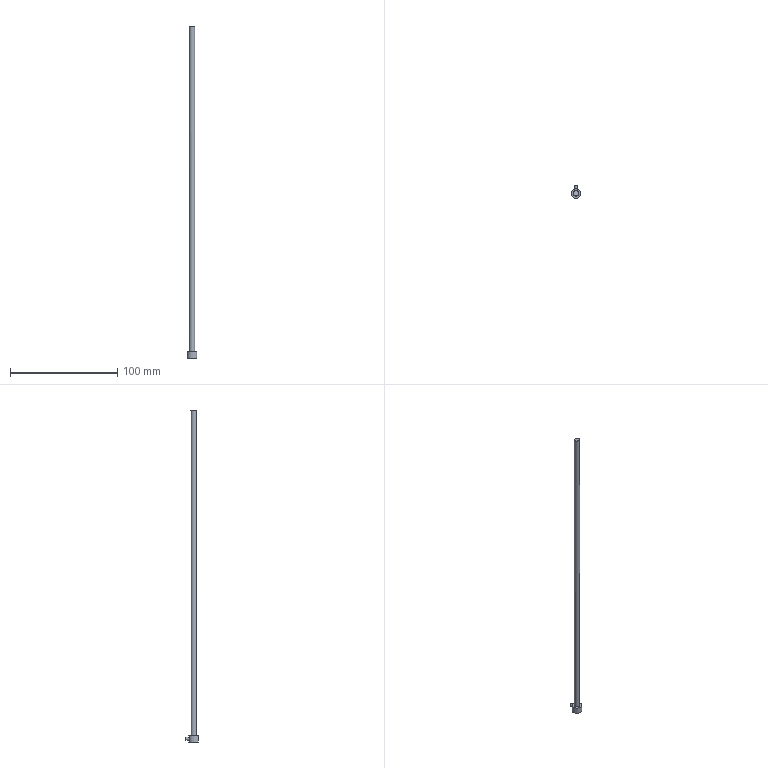Part | STEP file | E105-19-315 | 1 solid | 8 faces | box 9 x 12 x 309.26 mm | volume 6349 mm3 | cylinder 3 | plane 3 | spline 1 | cone 1 | commonest cylinder face diameters 3 x1 5 x1 9 x1
STEP:
#1=CARTESIAN_POINT('',(0.,0.,0.));
#2=DIRECTION('',(0.,0.,1.));
#3=DIRECTION('',(1.,0.,0.));
#4=AXIS2_PLACEMENT_3D('',#1,#2,#3);
#5=CARTESIAN_POINT('',(2.261,-1.066,308.914));
#6=VERTEX_POINT('',#5);
#7=CARTESIAN_POINT('',(-2.5,0.,308.912));
#8=VERTEX_POINT('',#7);
#9=CARTESIAN_POINT('',(2.261,-1.066,308.914));
#10=CARTESIAN_POINT('',(2.141,-1.321,308.963));
#11=CARTESIAN_POINT('',(1.975,-1.558,309.011));
#12=CARTESIAN_POINT('',(1.777,-1.759,309.053));
#13=CARTESIAN_POINT('',(1.578,-1.96,309.095));
#14=CARTESIAN_POINT('',(1.341,-2.129,309.134));
#15=CARTESIAN_POINT('',(1.085,-2.252,309.164));
#16=CARTESIAN_POINT('',(0.8317,-2.374,309.195));
#17=CARTESIAN_POINT('',(0.553,-2.454,309.22));
#18=CARTESIAN_POINT('',(0.2723,-2.485,309.236));
#19=CARTESIAN_POINT('',(-0.004267,-2.515,309.252));
#20=CARTESIAN_POINT('',(-0.2904,-2.499,309.26));
#21=CARTESIAN_POINT('',(-0.562,-2.436,309.26));
#22=CARTESIAN_POINT('',(-0.8311,-2.374,309.26));
#23=CARTESIAN_POINT('',(-1.093,-2.265,309.252));
#24=CARTESIAN_POINT('',(-1.327,-2.119,309.236));
#25=CARTESIAN_POINT('',(-1.561,-1.972,309.22));
#26=CARTESIAN_POINT('',(-1.772,-1.785,309.197));
#27=CARTESIAN_POINT('',(-1.944,-1.571,309.166));
#28=CARTESIAN_POINT('',(-2.118,-1.356,309.136));
#29=CARTESIAN_POINT('',(-2.257,-1.109,309.099));
#30=CARTESIAN_POINT('',(-2.351,-0.8505,309.057));
#31=CARTESIAN_POINT('',(-2.446,-0.588,309.014));
#32=CARTESIAN_POINT('',(-2.497,-0.3065,308.966));
#33=CARTESIAN_POINT('',(-2.5,-0.02854,308.917));
#34=CARTESIAN_POINT('',(-2.503,0.2536,308.866));
#35=CARTESIAN_POINT('',(-2.457,0.5396,308.813));
#36=CARTESIAN_POINT('',(-2.366,0.8063,308.76));
#37=CARTESIAN_POINT('',(-2.275,1.075,308.707));
#38=CARTESIAN_POINT('',(-2.134,1.332,308.654));
#39=CARTESIAN_POINT('',(-1.957,1.556,308.606));
#40=CARTESIAN_POINT('',(-1.78,1.778,308.558));
#41=CARTESIAN_POINT('',(-1.561,1.974,308.512));
#42=CARTESIAN_POINT('',(-1.318,2.124,308.474));
#43=CARTESIAN_POINT('',(-1.078,2.273,308.437));
#44=CARTESIAN_POINT('',(-0.8076,2.383,308.405));
#45=CARTESIAN_POINT('',(-0.53,2.443,308.383));
#46=CARTESIAN_POINT('',(-0.2575,2.502,308.361));
#47=CARTESIAN_POINT('',(0.02984,2.515,308.347));
#48=CARTESIAN_POINT('',(0.3074,2.481,308.343));
#49=CARTESIAN_POINT('',(0.5811,2.447,308.338));
#50=CARTESIAN_POINT('',(0.8529,2.366,308.343));
#51=CARTESIAN_POINT('',(1.1,2.245,308.356));
#52=CARTESIAN_POINT('',(1.347,2.124,308.369));
#53=CARTESIAN_POINT('',(1.576,1.96,308.391));
#54=CARTESIAN_POINT('',(1.769,1.766,308.42));
#55=CARTESIAN_POINT('',(1.964,1.571,308.449));
#56=CARTESIAN_POINT('',(2.128,1.341,308.485));
#57=CARTESIAN_POINT('',(2.248,1.094,308.526));
#58=CARTESIAN_POINT('',(2.37,0.8435,308.567));
#59=CARTESIAN_POINT('',(2.45,0.5692,308.614));
#60=CARTESIAN_POINT('',(2.483,0.2935,308.663));
#61=CARTESIAN_POINT('',(2.516,0.01345,308.712));
#62=CARTESIAN_POINT('',(2.501,-0.2757,308.765));
#63=CARTESIAN_POINT('',(2.439,-0.5505,308.816));
#64=CARTESIAN_POINT('',(2.399,-0.7277,308.849));
#65=CARTESIAN_POINT('',(2.339,-0.9016,308.882));
#66=CARTESIAN_POINT('',(2.261,-1.066,308.914));
#67=B_SPLINE_CURVE_WITH_KNOTS('',3,(#9,#10,#11,#12,#13,#14,#15,#16,#17,#18,#19,#20,#21,#22,#23,#24,#25,#26,#27,#28,#29,#30,#31,#32,#33,#34,#35,#36,#37,#38,#39,#40,#41,#42,#43,#44,#45,#46,#47,#48,#49,#50,#51,#52,#53,#54,#55,#56,#57,#58,#59,#60,#61,#62,#63,#64,#65,#66),.UNSPECIFIED.,.T.,.F.,(1,3,3,3,3,3,3,3,3,3,3,3,3,3,3,3,3,3,3,3,3,1),(-0.03486,0.,0.05436,0.1088,0.1626,0.2156,0.2682,0.3207,0.3737,0.4274,0.4819,0.537,0.592,0.6462,0.6995,0.752,0.8043,0.857,0.9107,0.9651,1.,1.054),.UNSPECIFIED.);
#68=CARTESIAN_POINT('',(0.,0.,106.));
#69=DIRECTION('',(0.,0.,-1.));
#70=DIRECTION('',(-1.,0.,0.));
#71=AXIS2_PLACEMENT_3D('',#68,#69,#70);
#72=CYLINDRICAL_SURFACE('',#71,2.5);
#73=CARTESIAN_POINT('',(3.582,-202.914));
#74=CARTESIAN_POINT('',(3.606,-202.924));
#75=CARTESIAN_POINT('',(3.653,-202.944));
#76=CARTESIAN_POINT('',(3.724,-202.974));
#77=CARTESIAN_POINT('',(3.795,-203.004));
#78=CARTESIAN_POINT('',(3.866,-203.032));
#79=CARTESIAN_POINT('',(3.937,-203.059));
#80=CARTESIAN_POINT('',(4.008,-203.085));
#81=CARTESIAN_POINT('',(4.08,-203.109));
#82=CARTESIAN_POINT('',(4.151,-203.132));
#83=CARTESIAN_POINT('',(4.223,-203.153));
#84=CARTESIAN_POINT('',(4.294,-203.173));
#85=CARTESIAN_POINT('',(4.366,-203.191));
#86=CARTESIAN_POINT('',(4.438,-203.207));
#87=CARTESIAN_POINT('',(4.509,-203.221));
#88=CARTESIAN_POINT('',(4.581,-203.233));
#89=CARTESIAN_POINT('',(4.653,-203.243));
#90=CARTESIAN_POINT('',(4.725,-203.25));
#91=CARTESIAN_POINT('',(4.797,-203.256));
#92=CARTESIAN_POINT('',(4.869,-203.259));
#93=CARTESIAN_POINT('',(4.941,-203.261));
#94=CARTESIAN_POINT('',(5.013,-203.259));
#95=CARTESIAN_POINT('',(5.085,-203.256));
#96=CARTESIAN_POINT('',(5.157,-203.25));
#97=CARTESIAN_POINT('',(5.229,-203.242));
#98=CARTESIAN_POINT('',(5.3,-203.232));
#99=CARTESIAN_POINT('',(5.372,-203.22));
#100=CARTESIAN_POINT('',(5.444,-203.206));
#101=CARTESIAN_POINT('',(5.516,-203.189));
#102=CARTESIAN_POINT('',(5.588,-203.171));
#103=CARTESIAN_POINT('',(5.659,-203.151));
#104=CARTESIAN_POINT('',(5.73,-203.129));
#105=CARTESIAN_POINT('',(5.802,-203.105));
#106=CARTESIAN_POINT('',(5.873,-203.08));
#107=CARTESIAN_POINT('',(5.944,-203.054));
#108=CARTESIAN_POINT('',(6.015,-203.026));
#109=CARTESIAN_POINT('',(6.087,-202.997));
#110=CARTESIAN_POINT('',(6.158,-202.967));
#111=CARTESIAN_POINT('',(6.229,-202.936));
#112=CARTESIAN_POINT('',(6.299,-202.904));
#113=CARTESIAN_POINT('',(6.37,-202.872));
#114=CARTESIAN_POINT('',(6.441,-202.84));
#115=CARTESIAN_POINT('',(6.512,-202.807));
#116=CARTESIAN_POINT('',(6.583,-202.774));
#117=CARTESIAN_POINT('',(6.653,-202.741));
#118=CARTESIAN_POINT('',(6.724,-202.708));
#119=CARTESIAN_POINT('',(6.795,-202.676));
#120=CARTESIAN_POINT('',(6.866,-202.644));
#121=CARTESIAN_POINT('',(6.937,-202.613));
#122=CARTESIAN_POINT('',(7.007,-202.584));
#123=CARTESIAN_POINT('',(7.079,-202.555));
#124=CARTESIAN_POINT('',(7.15,-202.527));
#125=CARTESIAN_POINT('',(7.221,-202.501));
#126=CARTESIAN_POINT('',(7.292,-202.476));
#127=CARTESIAN_POINT('',(7.363,-202.453));
#128=CARTESIAN_POINT('',(7.435,-202.432));
#129=CARTESIAN_POINT('',(7.507,-202.413));
#130=CARTESIAN_POINT('',(7.578,-202.395));
#131=CARTESIAN_POINT('',(7.65,-202.381));
#132=CARTESIAN_POINT('',(7.722,-202.368));
#133=CARTESIAN_POINT('',(7.794,-202.358));
#134=CARTESIAN_POINT('',(7.866,-202.35));
#135=CARTESIAN_POINT('',(7.938,-202.344));
#136=CARTESIAN_POINT('',(8.009,-202.341));
#137=CARTESIAN_POINT('',(8.081,-202.341));
#138=CARTESIAN_POINT('',(8.153,-202.343));
#139=CARTESIAN_POINT('',(8.226,-202.347));
#140=CARTESIAN_POINT('',(8.297,-202.354));
#141=CARTESIAN_POINT('',(8.369,-202.364));
#142=CARTESIAN_POINT('',(8.441,-202.375));
#143=CARTESIAN_POINT('',(8.513,-202.389));
#144=CARTESIAN_POINT('',(8.585,-202.406));
#145=CARTESIAN_POINT('',(8.656,-202.424));
#146=CARTESIAN_POINT('',(8.728,-202.444));
#147=CARTESIAN_POINT('',(8.799,-202.466));
#148=CARTESIAN_POINT('',(8.871,-202.49));
#149=CARTESIAN_POINT('',(8.942,-202.515));
#150=CARTESIAN_POINT('',(9.013,-202.541));
#151=CARTESIAN_POINT('',(9.084,-202.569));
#152=CARTESIAN_POINT('',(9.155,-202.598));
#153=CARTESIAN_POINT('',(9.227,-202.628));
#154=CARTESIAN_POINT('',(9.297,-202.658));
#155=CARTESIAN_POINT('',(9.368,-202.69));
#156=CARTESIAN_POINT('',(9.439,-202.721));
#157=CARTESIAN_POINT('',(9.51,-202.754));
#158=CARTESIAN_POINT('',(9.581,-202.786));
#159=CARTESIAN_POINT('',(9.651,-202.818));
#160=CARTESIAN_POINT('',(9.723,-202.85));
#161=CARTESIAN_POINT('',(9.794,-202.882));
#162=CARTESIAN_POINT('',(9.842,-202.903));
#163=CARTESIAN_POINT('',(9.865,-202.914));
#164=B_SPLINE_CURVE_WITH_KNOTS('',3,(#73,#74,#75,#76,#77,#78,#79,#80,#81,#82,#83,#84,#85,#86,#87,#88,#89,#90,#91,#92,#93,#94,#95,#96,#97,#98,#99,#100,#101,#102,#103,#104,#105,#106,#107,#108,#109,#110,#111,#112,#113,#114,#115,#116,#117,#118,#119,#120,#121,#122,#123,#124,#125,#126,#127,#128,#129,#130,#131,#132,#133,#134,#135,#136,#137,#138,#139,#140,#141,#142,#143,#144,#145,#146,#147,#148,#149,#150,#151,#152,#153,#154,#155,#156,#157,#158,#159,#160,#161,#162,#163),.UNSPECIFIED.,.F.,.F.,(4,1,1,1,1,1,1,1,1,1,1,1,1,1,1,1,1,1,1,1,1,1,1,1,1,1,1,1,1,1,1,1,1,1,1,1,1,1,1,1,1,1,1,1,1,1,1,1,1,1,1,1,1,1,1,1,1,1,1,1,1,1,1,1,1,1,1,1,1,1,1,1,1,1,1,1,1,1,1,1,1,1,1,1,1,1,1,1,4),(0.,0.01136,0.02273,0.03409,0.04545,0.05682,0.06818,0.07955,0.09091,0.1023,0.1136,0.125,0.1364,0.1477,0.1591,0.1705,0.1818,0.1932,0.2045,0.2159,0.2273,0.2386,0.25,0.2614,0.2727,0.2841,0.2955,0.3068,0.3182,0.3295,0.3409,0.3523,0.3636,0.375,0.3864,0.3977,0.4091,0.4205,0.4318,0.4432,0.4545,0.4659,0.4773,0.4886,0.5,0.5114,0.5227,0.5341,0.5455,0.5568,0.5682,0.5795,0.5909,0.6023,0.6136,0.625,0.6364,0.6477,0.6591,0.6705,0.6818,0.6932,0.7045,0.7159,0.7273,0.7386,0.75,0.7614,0.7727,0.7841,0.7955,0.8068,0.8182,0.8295,0.8409,0.8523,0.8636,0.875,0.8864,0.8977,0.9091,0.9205,0.9318,0.9432,0.9545,0.9659,0.9773,0.9886,1.),.QUASI_UNIFORM_KNOTS.);
#165=(GEOMETRIC_REPRESENTATION_CONTEXT(2)PARAMETRIC_REPRESENTATION_CONTEXT()REPRESENTATION_CONTEXT('',''));
#166=DEFINITIONAL_REPRESENTATION('',(#164),#165);
#167=PCURVE('',#72,#166);
#168=CARTESIAN_POINT('',(-6.353,3.18,308.471));
#169=CARTESIAN_POINT('',(-6.352,0.7834,308.933));
#170=CARTESIAN_POINT('',(-6.351,-1.62,309.36));
#171=CARTESIAN_POINT('',(-6.35,-4.031,309.75));
#172=CARTESIAN_POINT('',(-1.324,3.172,308.275));
#173=CARTESIAN_POINT('',(-1.323,0.7765,308.737));
#174=CARTESIAN_POINT('',(-1.322,-1.626,309.164));
#175=CARTESIAN_POINT('',(-1.32,-4.035,309.555));
#176=CARTESIAN_POINT('',(3.706,3.167,308.077));
#177=CARTESIAN_POINT('',(3.707,0.7722,308.54));
#178=CARTESIAN_POINT('',(3.708,-1.629,308.967));
#179=CARTESIAN_POINT('',(3.709,-4.037,309.359));
#180=CARTESIAN_POINT('',(8.735,3.164,307.878));
#181=CARTESIAN_POINT('',(8.736,0.7703,308.342));
#182=CARTESIAN_POINT('',(8.737,-1.63,308.769));
#183=CARTESIAN_POINT('',(8.738,-4.037,309.161));
#184=B_SPLINE_SURFACE_WITH_KNOTS('',3,3,((#168,#169,#170,#171),(#172,#173,#174,#175),(#176,#177,#178,#179),(#180,#181,#182,#183)),.UNSPECIFIED.,.F.,.F.,.F.,(4,4),(4,4),(0.,1.),(0.,1.),.PIECEWISE_BEZIER_KNOTS.);
#185=CARTESIAN_POINT('',(0.5708,0.5885));
#186=CARTESIAN_POINT('',(0.5694,0.5948));
#187=CARTESIAN_POINT('',(0.5663,0.6074));
#188=CARTESIAN_POINT('',(0.5612,0.6256));
#189=CARTESIAN_POINT('',(0.5555,0.6432));
#190=CARTESIAN_POINT('',(0.5494,0.66));
#191=CARTESIAN_POINT('',(0.5427,0.676));
#192=CARTESIAN_POINT('',(0.5357,0.6911));
#193=CARTESIAN_POINT('',(0.5281,0.7053));
#194=CARTESIAN_POINT('',(0.5202,0.7185));
#195=CARTESIAN_POINT('',(0.5118,0.7307));
#196=CARTESIAN_POINT('',(0.5032,0.7419));
#197=CARTESIAN_POINT('',(0.4942,0.7519));
#198=CARTESIAN_POINT('',(0.485,0.7607));
#199=CARTESIAN_POINT('',(0.4754,0.7683));
#200=CARTESIAN_POINT('',(0.4657,0.7747));
#201=CARTESIAN_POINT('',(0.4557,0.7799));
#202=CARTESIAN_POINT('',(0.4457,0.7837));
#203=CARTESIAN_POINT('',(0.4356,0.7863));
#204=CARTESIAN_POINT('',(0.4254,0.7875));
#205=CARTESIAN_POINT('',(0.4151,0.7874));
#206=CARTESIAN_POINT('',(0.4049,0.786));
#207=CARTESIAN_POINT('',(0.3947,0.7833));
#208=CARTESIAN_POINT('',(0.3847,0.7794));
#209=CARTESIAN_POINT('',(0.3748,0.7741));
#210=CARTESIAN_POINT('',(0.365,0.7675));
#211=CARTESIAN_POINT('',(0.3555,0.7596));
#212=CARTESIAN_POINT('',(0.3462,0.7506));
#213=CARTESIAN_POINT('',(0.3372,0.7404));
#214=CARTESIAN_POINT('',(0.3286,0.7291));
#215=CARTESIAN_POINT('',(0.3203,0.7166));
#216=CARTESIAN_POINT('',(0.3123,0.7031));
#217=CARTESIAN_POINT('',(0.3048,0.6886));
#218=CARTESIAN_POINT('',(0.2978,0.6733));
#219=CARTESIAN_POINT('',(0.2912,0.6571));
#220=CARTESIAN_POINT('',(0.2851,0.6401));
#221=CARTESIAN_POINT('',(0.2796,0.6223));
#222=CARTESIAN_POINT('',(0.2745,0.6038));
#223=CARTESIAN_POINT('',(0.27,0.5847));
#224=CARTESIAN_POINT('',(0.2661,0.5652));
#225=CARTESIAN_POINT('',(0.2628,0.5452));
#226=CARTESIAN_POINT('',(0.2601,0.5249));
#227=CARTESIAN_POINT('',(0.2579,0.5041));
#228=CARTESIAN_POINT('',(0.2564,0.4832));
#229=CARTESIAN_POINT('',(0.2555,0.4621));
#230=CARTESIAN_POINT('',(0.2553,0.4481));
#231=CARTESIAN_POINT('',(0.2553,0.4411));
#232=B_SPLINE_CURVE_WITH_KNOTS('',3,(#185,#186,#187,#188,#189,#190,#191,#192,#193,#194,#195,#196,#197,#198,#199,#200,#201,#202,#203,#204,#205,#206,#207,#208,#209,#210,#211,#212,#213,#214,#215,#216,#217,#218,#219,#220,#221,#222,#223,#224,#225,#226,#227,#228,#229,#230,#231),.UNSPECIFIED.,.F.,.F.,(4,1,1,1,1,1,1,1,1,1,1,1,1,1,1,1,1,1,1,1,1,1,1,1,1,1,1,1,1,1,1,1,1,1,1,1,1,1,1,1,1,1,1,1,4),(0.,0.009755,0.01951,0.02927,0.03902,0.04878,0.05853,0.06829,0.07804,0.0878,0.09755,0.1073,0.1171,0.1268,0.1366,0.1463,0.1561,0.1658,0.1756,0.1853,0.1951,0.2049,0.2146,0.2244,0.2341,0.2439,0.2536,0.2634,0.2731,0.2829,0.2927,0.3024,0.3122,0.3219,0.3317,0.3414,0.3512,0.3609,0.3707,0.3804,0.3902,0.4,0.4097,0.4195,0.4292),.QUASI_UNIFORM_KNOTS.);
#233=(GEOMETRIC_REPRESENTATION_CONTEXT(2)PARAMETRIC_REPRESENTATION_CONTEXT()REPRESENTATION_CONTEXT('',''));
#234=DEFINITIONAL_REPRESENTATION('',(#232),#233);
#235=PCURVE('',#184,#234);
#236=SURFACE_CURVE('',#67,(#167,#235),.PCURVE_S1.);
#237=EDGE_CURVE('',#6,#8,#236,.T.);
#238=ORIENTED_EDGE('',*,*,#237,.T.);
#239=CARTESIAN_POINT('',(-2.5,0.,6.));
#240=VERTEX_POINT('',#239);
#241=CARTESIAN_POINT('',(-2.5,0.,308.912));
#242=CARTESIAN_POINT('',(-2.5,0.,6.));
#243=B_SPLINE_CURVE_WITH_KNOTS('',1,(#241,#242),.UNSPECIFIED.,.F.,.F.,(2,2),(-202.912,100.),.PIECEWISE_BEZIER_KNOTS.);
#244=CARTESIAN_POINT('',(6.283,0.));
#245=DIRECTION('',(0.,1.));
#246=VECTOR('',#245,1.);
#247=LINE('',#244,#246);
#248=(GEOMETRIC_REPRESENTATION_CONTEXT(2)PARAMETRIC_REPRESENTATION_CONTEXT()REPRESENTATION_CONTEXT('',''));
#249=DEFINITIONAL_REPRESENTATION('',(#247),#248);
#250=PCURVE('',#72,#249);
#251=CARTESIAN_POINT('',(0.,0.));
#252=DIRECTION('',(0.,1.));
#253=VECTOR('',#252,1.);
#254=LINE('',#251,#253);
#255=(GEOMETRIC_REPRESENTATION_CONTEXT(2)PARAMETRIC_REPRESENTATION_CONTEXT()REPRESENTATION_CONTEXT('',''));
#256=DEFINITIONAL_REPRESENTATION('',(#254),#255);
#257=PCURVE('',#72,#256);
#258=SEAM_CURVE('',#243,(#250,#257),.PCURVE_S1.);
#259=EDGE_CURVE('',#8,#240,#258,.T.);
#260=ORIENTED_EDGE('',*,*,#259,.T.);
#261=CARTESIAN_POINT('',(0.,0.,6.));
#262=DIRECTION('',(0.,0.,-1.));
#263=DIRECTION('',(-1.,0.,0.));
#264=AXIS2_PLACEMENT_3D('',#261,#262,#263);
#265=CIRCLE('',#264,2.5);
#266=CARTESIAN_POINT('',(0.,100.));
#267=DIRECTION('',(1.,0.));
#268=VECTOR('',#267,1.);
#269=LINE('',#266,#268);
#270=(GEOMETRIC_REPRESENTATION_CONTEXT(2)PARAMETRIC_REPRESENTATION_CONTEXT()REPRESENTATION_CONTEXT('',''));
#271=DEFINITIONAL_REPRESENTATION('',(#269),#270);
#272=PCURVE('',#72,#271);
#273=CARTESIAN_POINT('',(0.,0.,6.));
#274=DIRECTION('',(0.,0.,-1.));
#275=DIRECTION('',(1.,0.,0.));
#276=AXIS2_PLACEMENT_3D('',#273,#274,#275);
#277=PLANE('',#276);
#278=CARTESIAN_POINT('',(0.,0.));
#279=DIRECTION('',(-1.,0.));
#280=AXIS2_PLACEMENT_2D('',#278,#279);
#281=CIRCLE('',#280,2.5);
#282=(GEOMETRIC_REPRESENTATION_CONTEXT(2)PARAMETRIC_REPRESENTATION_CONTEXT()REPRESENTATION_CONTEXT('',''));
#283=DEFINITIONAL_REPRESENTATION('',(#281),#282);
#284=PCURVE('',#277,#283);
#285=SURFACE_CURVE('',#265,(#272,#284),.PCURVE_S1.);
#286=EDGE_CURVE('',#240,#240,#285,.T.);
#287=ORIENTED_EDGE('',*,*,#286,.F.);
#288=ORIENTED_EDGE('',*,*,#259,.F.);
#289=CARTESIAN_POINT('',(2.261,-1.066,308.914));
#290=CARTESIAN_POINT('',(2.141,-1.321,308.963));
#291=CARTESIAN_POINT('',(1.975,-1.558,309.011));
#292=CARTESIAN_POINT('',(1.777,-1.759,309.053));
#293=CARTESIAN_POINT('',(1.578,-1.96,309.095));
#294=CARTESIAN_POINT('',(1.341,-2.129,309.134));
#295=CARTESIAN_POINT('',(1.085,-2.252,309.164));
#296=CARTESIAN_POINT('',(0.8317,-2.374,309.195));
#297=CARTESIAN_POINT('',(0.553,-2.454,309.22));
#298=CARTESIAN_POINT('',(0.2723,-2.485,309.236));
#299=CARTESIAN_POINT('',(-0.004267,-2.515,309.252));
#300=CARTESIAN_POINT('',(-0.2904,-2.499,309.26));
#301=CARTESIAN_POINT('',(-0.562,-2.436,309.26));
#302=CARTESIAN_POINT('',(-0.8311,-2.374,309.26));
#303=CARTESIAN_POINT('',(-1.093,-2.265,309.252));
#304=CARTESIAN_POINT('',(-1.327,-2.119,309.236));
#305=CARTESIAN_POINT('',(-1.561,-1.972,309.22));
#306=CARTESIAN_POINT('',(-1.772,-1.785,309.197));
#307=CARTESIAN_POINT('',(-1.944,-1.571,309.166));
#308=CARTESIAN_POINT('',(-2.118,-1.356,309.136));
#309=CARTESIAN_POINT('',(-2.257,-1.109,309.099));
#310=CARTESIAN_POINT('',(-2.351,-0.8505,309.057));
#311=CARTESIAN_POINT('',(-2.446,-0.588,309.014));
#312=CARTESIAN_POINT('',(-2.497,-0.3065,308.966));
#313=CARTESIAN_POINT('',(-2.5,-0.02854,308.917));
#314=CARTESIAN_POINT('',(-2.503,0.2536,308.866));
#315=CARTESIAN_POINT('',(-2.457,0.5396,308.813));
#316=CARTESIAN_POINT('',(-2.366,0.8063,308.76));
#317=CARTESIAN_POINT('',(-2.275,1.075,308.707));
#318=CARTESIAN_POINT('',(-2.134,1.332,308.654));
#319=CARTESIAN_POINT('',(-1.957,1.556,308.606));
#320=CARTESIAN_POINT('',(-1.78,1.778,308.558));
#321=CARTESIAN_POINT('',(-1.561,1.974,308.512));
#322=CARTESIAN_POINT('',(-1.318,2.124,308.474));
#323=CARTESIAN_POINT('',(-1.078,2.273,308.437));
#324=CARTESIAN_POINT('',(-0.8076,2.383,308.405));
#325=CARTESIAN_POINT('',(-0.53,2.443,308.383));
#326=CARTESIAN_POINT('',(-0.2575,2.502,308.361));
#327=CARTESIAN_POINT('',(0.02984,2.515,308.347));
#328=CARTESIAN_POINT('',(0.3074,2.481,308.343));
#329=CARTESIAN_POINT('',(0.5811,2.447,308.338));
#330=CARTESIAN_POINT('',(0.8529,2.366,308.343));
#331=CARTESIAN_POINT('',(1.1,2.245,308.356));
#332=CARTESIAN_POINT('',(1.347,2.124,308.369));
#333=CARTESIAN_POINT('',(1.576,1.96,308.391));
#334=CARTESIAN_POINT('',(1.769,1.766,308.42));
#335=CARTESIAN_POINT('',(1.964,1.571,308.449));
#336=CARTESIAN_POINT('',(2.128,1.341,308.485));
#337=CARTESIAN_POINT('',(2.248,1.094,308.526));
#338=CARTESIAN_POINT('',(2.37,0.8435,308.567));
#339=CARTESIAN_POINT('',(2.45,0.5692,308.614));
#340=CARTESIAN_POINT('',(2.483,0.2935,308.663));
#341=CARTESIAN_POINT('',(2.516,0.01345,308.712));
#342=CARTESIAN_POINT('',(2.501,-0.2757,308.765));
#343=CARTESIAN_POINT('',(2.439,-0.5505,308.816));
#344=CARTESIAN_POINT('',(2.399,-0.7277,308.849));
#345=CARTESIAN_POINT('',(2.339,-0.9016,308.882));
#346=CARTESIAN_POINT('',(2.261,-1.066,308.914));
#347=B_SPLINE_CURVE_WITH_KNOTS('',3,(#289,#290,#291,#292,#293,#294,#295,#296,#297,#298,#299,#300,#301,#302,#303,#304,#305,#306,#307,#308,#309,#310,#311,#312,#313,#314,#315,#316,#317,#318,#319,#320,#321,#322,#323,#324,#325,#326,#327,#328,#329,#330,#331,#332,#333,#334,#335,#336,#337,#338,#339,#340,#341,#342,#343,#344,#345,#346),.UNSPECIFIED.,.T.,.F.,(1,3,3,3,3,3,3,3,3,3,3,3,3,3,3,3,3,3,3,3,3,1),(-0.03486,0.,0.05436,0.1088,0.1626,0.2156,0.2682,0.3207,0.3737,0.4274,0.4819,0.537,0.592,0.6462,0.6995,0.752,0.8043,0.857,0.9107,0.9651,1.,1.054),.UNSPECIFIED.);
#348=CARTESIAN_POINT('',(-2.701,-202.914));
#349=CARTESIAN_POINT('',(-2.677,-202.924));
#350=CARTESIAN_POINT('',(-2.63,-202.944));
#351=CARTESIAN_POINT('',(-2.559,-202.974));
#352=CARTESIAN_POINT('',(-2.488,-203.004));
#353=CARTESIAN_POINT('',(-2.417,-203.032));
#354=CARTESIAN_POINT('',(-2.346,-203.059));
#355=CARTESIAN_POINT('',(-2.275,-203.085));
#356=CARTESIAN_POINT('',(-2.203,-203.109));
#357=CARTESIAN_POINT('',(-2.132,-203.132));
#358=CARTESIAN_POINT('',(-2.06,-203.153));
#359=CARTESIAN_POINT('',(-1.989,-203.173));
#360=CARTESIAN_POINT('',(-1.918,-203.191));
#361=CARTESIAN_POINT('',(-1.846,-203.207));
#362=CARTESIAN_POINT('',(-1.774,-203.221));
#363=CARTESIAN_POINT('',(-1.702,-203.233));
#364=CARTESIAN_POINT('',(-1.63,-203.243));
#365=CARTESIAN_POINT('',(-1.558,-203.25));
#366=CARTESIAN_POINT('',(-1.486,-203.256));
#367=CARTESIAN_POINT('',(-1.414,-203.259));
#368=CARTESIAN_POINT('',(-1.342,-203.261));
#369=CARTESIAN_POINT('',(-1.271,-203.259));
#370=CARTESIAN_POINT('',(-1.198,-203.256));
#371=CARTESIAN_POINT('',(-1.126,-203.25));
#372=CARTESIAN_POINT('',(-1.054,-203.242));
#373=CARTESIAN_POINT('',(-0.9828,-203.232));
#374=CARTESIAN_POINT('',(-0.9109,-203.22));
#375=CARTESIAN_POINT('',(-0.839,-203.206));
#376=CARTESIAN_POINT('',(-0.7671,-203.189));
#377=CARTESIAN_POINT('',(-0.6955,-203.171));
#378=CARTESIAN_POINT('',(-0.6243,-203.151));
#379=CARTESIAN_POINT('',(-0.5527,-203.129));
#380=CARTESIAN_POINT('',(-0.4812,-203.105));
#381=CARTESIAN_POINT('',(-0.4097,-203.08));
#382=CARTESIAN_POINT('',(-0.3388,-203.054));
#383=CARTESIAN_POINT('',(-0.2678,-203.026));
#384=CARTESIAN_POINT('',(-0.1966,-202.997));
#385=CARTESIAN_POINT('',(-0.1254,-202.967));
#386=CARTESIAN_POINT('',(-0.05444,-202.936));
#387=CARTESIAN_POINT('',(0.01607,-202.904));
#388=CARTESIAN_POINT('',(0.08688,-202.872));
#389=CARTESIAN_POINT('',(0.1578,-202.84));
#390=CARTESIAN_POINT('',(0.2288,-202.807));
#391=CARTESIAN_POINT('',(0.2995,-202.774));
#392=CARTESIAN_POINT('',(0.3699,-202.741));
#393=CARTESIAN_POINT('',(0.4408,-202.708));
#394=CARTESIAN_POINT('',(0.5117,-202.676));
#395=CARTESIAN_POINT('',(0.5827,-202.644));
#396=CARTESIAN_POINT('',(0.6536,-202.613));
#397=CARTESIAN_POINT('',(0.7242,-202.584));
#398=CARTESIAN_POINT('',(0.7953,-202.555));
#399=CARTESIAN_POINT('',(0.8666,-202.527));
#400=CARTESIAN_POINT('',(0.9379,-202.501));
#401=CARTESIAN_POINT('',(1.009,-202.476));
#402=CARTESIAN_POINT('',(1.08,-202.453));
#403=CARTESIAN_POINT('',(1.152,-202.432));
#404=CARTESIAN_POINT('',(1.224,-202.413));
#405=CARTESIAN_POINT('',(1.295,-202.395));
#406=CARTESIAN_POINT('',(1.367,-202.381));
#407=CARTESIAN_POINT('',(1.438,-202.368));
#408=CARTESIAN_POINT('',(1.51,-202.358));
#409=CARTESIAN_POINT('',(1.582,-202.35));
#410=CARTESIAN_POINT('',(1.654,-202.344));
#411=CARTESIAN_POINT('',(1.726,-202.341));
#412=CARTESIAN_POINT('',(1.798,-202.341));
#413=CARTESIAN_POINT('',(1.87,-202.343));
#414=CARTESIAN_POINT('',(1.942,-202.347));
#415=CARTESIAN_POINT('',(2.014,-202.354));
#416=CARTESIAN_POINT('',(2.086,-202.364));
#417=CARTESIAN_POINT('',(2.158,-202.375));
#418=CARTESIAN_POINT('',(2.23,-202.389));
#419=CARTESIAN_POINT('',(2.302,-202.406));
#420=CARTESIAN_POINT('',(2.373,-202.424));
#421=CARTESIAN_POINT('',(2.444,-202.444));
#422=CARTESIAN_POINT('',(2.516,-202.466));
#423=CARTESIAN_POINT('',(2.588,-202.49));
#424=CARTESIAN_POINT('',(2.659,-202.515));
#425=CARTESIAN_POINT('',(2.73,-202.541));
#426=CARTESIAN_POINT('',(2.801,-202.569));
#427=CARTESIAN_POINT('',(2.872,-202.598));
#428=CARTESIAN_POINT('',(2.943,-202.628));
#429=CARTESIAN_POINT('',(3.014,-202.658));
#430=CARTESIAN_POINT('',(3.085,-202.69));
#431=CARTESIAN_POINT('',(3.156,-202.721));
#432=CARTESIAN_POINT('',(3.227,-202.754));
#433=CARTESIAN_POINT('',(3.298,-202.786));
#434=CARTESIAN_POINT('',(3.368,-202.818));
#435=CARTESIAN_POINT('',(3.44,-202.85));
#436=CARTESIAN_POINT('',(3.511,-202.882));
#437=CARTESIAN_POINT('',(3.558,-202.903));
#438=CARTESIAN_POINT('',(3.582,-202.914));
#439=B_SPLINE_CURVE_WITH_KNOTS('',3,(#348,#349,#350,#351,#352,#353,#354,#355,#356,#357,#358,#359,#360,#361,#362,#363,#364,#365,#366,#367,#368,#369,#370,#371,#372,#373,#374,#375,#376,#377,#378,#379,#380,#381,#382,#383,#384,#385,#386,#387,#388,#389,#390,#391,#392,#393,#394,#395,#396,#397,#398,#399,#400,#401,#402,#403,#404,#405,#406,#407,#408,#409,#410,#411,#412,#413,#414,#415,#416,#417,#418,#419,#420,#421,#422,#423,#424,#425,#426,#427,#428,#429,#430,#431,#432,#433,#434,#435,#436,#437,#438),.UNSPECIFIED.,.F.,.F.,(4,1,1,1,1,1,1,1,1,1,1,1,1,1,1,1,1,1,1,1,1,1,1,1,1,1,1,1,1,1,1,1,1,1,1,1,1,1,1,1,1,1,1,1,1,1,1,1,1,1,1,1,1,1,1,1,1,1,1,1,1,1,1,1,1,1,1,1,1,1,1,1,1,1,1,1,1,1,1,1,1,1,1,1,1,1,1,1,4),(0.,0.01136,0.02273,0.03409,0.04545,0.05682,0.06818,0.07955,0.09091,0.1023,0.1136,0.125,0.1364,0.1477,0.1591,0.1705,0.1818,0.1932,0.2045,0.2159,0.2273,0.2386,0.25,0.2614,0.2727,0.2841,0.2955,0.3068,0.3182,0.3295,0.3409,0.3523,0.3636,0.375,0.3864,0.3977,0.4091,0.4205,0.4318,0.4432,0.4545,0.4659,0.4773,0.4886,0.5,0.5114,0.5227,0.5341,0.5455,0.5568,0.5682,0.5795,0.5909,0.6023,0.6136,0.625,0.6364,0.6477,0.6591,0.6705,0.6818,0.6932,0.7045,0.7159,0.7273,0.7386,0.75,0.7614,0.7727,0.7841,0.7955,0.8068,0.8182,0.8295,0.8409,0.8523,0.8636,0.875,0.8864,0.8977,0.9091,0.9205,0.9318,0.9432,0.9545,0.9659,0.9773,0.9886,1.),.QUASI_UNIFORM_KNOTS.);
#440=(GEOMETRIC_REPRESENTATION_CONTEXT(2)PARAMETRIC_REPRESENTATION_CONTEXT()REPRESENTATION_CONTEXT('',''));
#441=DEFINITIONAL_REPRESENTATION('',(#439),#440);
#442=PCURVE('',#72,#441);
#443=CARTESIAN_POINT('',(0.2553,0.4411));
#444=CARTESIAN_POINT('',(0.2553,0.4318));
#445=CARTESIAN_POINT('',(0.2557,0.4131));
#446=CARTESIAN_POINT('',(0.2573,0.3852));
#447=CARTESIAN_POINT('',(0.26,0.3576));
#448=CARTESIAN_POINT('',(0.2637,0.3307));
#449=CARTESIAN_POINT('',(0.2685,0.3046));
#450=CARTESIAN_POINT('',(0.2743,0.2791));
#451=CARTESIAN_POINT('',(0.281,0.2548));
#452=CARTESIAN_POINT('',(0.2886,0.2316));
#453=CARTESIAN_POINT('',(0.2971,0.2099));
#454=CARTESIAN_POINT('',(0.3065,0.1896));
#455=CARTESIAN_POINT('',(0.3166,0.1709));
#456=CARTESIAN_POINT('',(0.3275,0.1539));
#457=CARTESIAN_POINT('',(0.3389,0.139));
#458=CARTESIAN_POINT('',(0.3509,0.1259));
#459=CARTESIAN_POINT('',(0.3634,0.1149));
#460=CARTESIAN_POINT('',(0.3763,0.106));
#461=CARTESIAN_POINT('',(0.3895,0.09947));
#462=CARTESIAN_POINT('',(0.4029,0.0952));
#463=CARTESIAN_POINT('',(0.4165,0.09322));
#464=CARTESIAN_POINT('',(0.4302,0.09356));
#465=CARTESIAN_POINT('',(0.4437,0.09624));
#466=CARTESIAN_POINT('',(0.4571,0.1013));
#467=CARTESIAN_POINT('',(0.4703,0.1087));
#468=CARTESIAN_POINT('',(0.4832,0.1182));
#469=CARTESIAN_POINT('',(0.4955,0.1299));
#470=CARTESIAN_POINT('',(0.5074,0.1438));
#471=CARTESIAN_POINT('',(0.5187,0.1596));
#472=CARTESIAN_POINT('',(0.5294,0.1774));
#473=CARTESIAN_POINT('',(0.5393,0.1967));
#474=CARTESIAN_POINT('',(0.5483,0.2177));
#475=CARTESIAN_POINT('',(0.5566,0.2403));
#476=CARTESIAN_POINT('',(0.5639,0.2641));
#477=CARTESIAN_POINT('',(0.5703,0.2889));
#478=CARTESIAN_POINT('',(0.5756,0.3148));
#479=CARTESIAN_POINT('',(0.58,0.3415));
#480=CARTESIAN_POINT('',(0.5833,0.3689));
#481=CARTESIAN_POINT('',(0.5855,0.3966));
#482=CARTESIAN_POINT('',(0.5867,0.4245));
#483=CARTESIAN_POINT('',(0.5867,0.4527));
#484=CARTESIAN_POINT('',(0.5857,0.4808));
#485=CARTESIAN_POINT('',(0.5836,0.5084));
#486=CARTESIAN_POINT('',(0.5805,0.5358));
#487=CARTESIAN_POINT('',(0.5762,0.5627));
#488=CARTESIAN_POINT('',(0.5727,0.58));
#489=CARTESIAN_POINT('',(0.5708,0.5885));
#490=B_SPLINE_CURVE_WITH_KNOTS('',3,(#443,#444,#445,#446,#447,#448,#449,#450,#451,#452,#453,#454,#455,#456,#457,#458,#459,#460,#461,#462,#463,#464,#465,#466,#467,#468,#469,#470,#471,#472,#473,#474,#475,#476,#477,#478,#479,#480,#481,#482,#483,#484,#485,#486,#487,#488,#489),.UNSPECIFIED.,.F.,.F.,(4,1,1,1,1,1,1,1,1,1,1,1,1,1,1,1,1,1,1,1,1,1,1,1,1,1,1,1,1,1,1,1,1,1,1,1,1,1,1,1,1,1,1,1,4),(0.4292,0.4422,0.4552,0.4681,0.4811,0.4941,0.5071,0.52,0.533,0.546,0.5589,0.5719,0.5849,0.5979,0.6108,0.6238,0.6368,0.6498,0.6627,0.6757,0.6887,0.7016,0.7146,0.7276,0.7406,0.7535,0.7665,0.7795,0.7924,0.8054,0.8184,0.8314,0.8443,0.8573,0.8703,0.8833,0.8962,0.9092,0.9222,0.9351,0.9481,0.9611,0.9741,0.987,1.),.QUASI_UNIFORM_KNOTS.);
#491=(GEOMETRIC_REPRESENTATION_CONTEXT(2)PARAMETRIC_REPRESENTATION_CONTEXT()REPRESENTATION_CONTEXT('',''));
#492=DEFINITIONAL_REPRESENTATION('',(#490),#491);
#493=PCURVE('',#184,#492);
#494=SURFACE_CURVE('',#347,(#442,#493),.PCURVE_S1.);
#495=EDGE_CURVE('',#8,#6,#494,.T.);
#496=ORIENTED_EDGE('',*,*,#495,.T.);
#497=EDGE_LOOP('',(#238,#260,#287,#288,#496));
#498=FACE_BOUND('',#497,.T.);
#499=ADVANCED_FACE('',(#498),#72,.T.);
#500=ORIENTED_EDGE('',*,*,#495,.T.);
#501=ORIENTED_EDGE('',*,*,#237,.T.);
#502=EDGE_LOOP('',(#500,#501));
#503=FACE_BOUND('',#502,.F.);
#504=ADVANCED_FACE('',(#503),#184,.F.);
#505=CARTESIAN_POINT('',(-4.5,0.,6.));
#506=VERTEX_POINT('',#505);
#507=CARTESIAN_POINT('',(0.,0.,6.));
#508=DIRECTION('',(0.,0.,-1.));
#509=DIRECTION('',(-1.,0.,0.));
#510=AXIS2_PLACEMENT_3D('',#507,#508,#509);
#511=CIRCLE('',#510,4.5);
#512=CARTESIAN_POINT('',(0.,0.));
#513=DIRECTION('',(-1.,0.));
#514=AXIS2_PLACEMENT_2D('',#512,#513);
#515=CIRCLE('',#514,4.5);
#516=(GEOMETRIC_REPRESENTATION_CONTEXT(2)PARAMETRIC_REPRESENTATION_CONTEXT()REPRESENTATION_CONTEXT('',''));
#517=DEFINITIONAL_REPRESENTATION('',(#515),#516);
#518=PCURVE('',#277,#517);
#519=CARTESIAN_POINT('',(0.,0.,-21.));
#520=DIRECTION('',(0.,0.,1.));
#521=DIRECTION('',(-1.,0.,0.));
#522=AXIS2_PLACEMENT_3D('',#519,#520,#521);
#523=CYLINDRICAL_SURFACE('',#522,4.5);
#524=CARTESIAN_POINT('',(6.283,27.));
#525=DIRECTION('',(-1.,0.));
#526=VECTOR('',#525,1.);
#527=LINE('',#524,#526);
#528=(GEOMETRIC_REPRESENTATION_CONTEXT(2)PARAMETRIC_REPRESENTATION_CONTEXT()REPRESENTATION_CONTEXT('',''));
#529=DEFINITIONAL_REPRESENTATION('',(#527),#528);
#530=PCURVE('',#523,#529);
#531=SURFACE_CURVE('',#511,(#518,#530),.PCURVE_S1.);
#532=EDGE_CURVE('',#506,#506,#531,.T.);
#533=ORIENTED_EDGE('',*,*,#532,.F.);
#534=EDGE_LOOP('',(#533));
#535=FACE_BOUND('',#534,.T.);
#536=ORIENTED_EDGE('',*,*,#286,.T.);
#537=EDGE_LOOP('',(#536));
#538=FACE_BOUND('',#537,.T.);
#539=ADVANCED_FACE('',(#535,#538),#277,.F.);
#540=CARTESIAN_POINT('',(4.5,0.,0.));
#541=VERTEX_POINT('',#540);
#542=CARTESIAN_POINT('',(-4.5,0.,0.));
#543=VERTEX_POINT('',#542);
#544=CARTESIAN_POINT('',(0.,0.,0.));
#545=DIRECTION('',(0.,0.,1.));
#546=DIRECTION('',(1.,0.,0.));
#547=AXIS2_PLACEMENT_3D('',#544,#545,#546);
#548=CIRCLE('',#547,4.5);
#549=CARTESIAN_POINT('',(3.142,21.));
#550=DIRECTION('',(1.,0.));
#551=VECTOR('',#550,1.);
#552=LINE('',#549,#551);
#553=(GEOMETRIC_REPRESENTATION_CONTEXT(2)PARAMETRIC_REPRESENTATION_CONTEXT()REPRESENTATION_CONTEXT('',''));
#554=DEFINITIONAL_REPRESENTATION('',(#552),#553);
#555=PCURVE('',#523,#554);
#556=CARTESIAN_POINT('',(320.,-1000.,0.));
#557=DIRECTION('',(0.,0.,1.));
#558=DIRECTION('',(-1.,0.,0.));
#559=AXIS2_PLACEMENT_3D('',#556,#557,#558);
#560=PLANE('',#559);
#561=CARTESIAN_POINT('',(320.,-1000.));
#562=DIRECTION('',(-1.,0.));
#563=AXIS2_PLACEMENT_2D('',#561,#562);
#564=CIRCLE('',#563,4.5);
#565=(GEOMETRIC_REPRESENTATION_CONTEXT(2)PARAMETRIC_REPRESENTATION_CONTEXT()REPRESENTATION_CONTEXT('',''));
#566=DEFINITIONAL_REPRESENTATION('',(#564),#565);
#567=PCURVE('',#560,#566);
#568=SURFACE_CURVE('',#548,(#555,#567),.PCURVE_S1.);
#569=EDGE_CURVE('',#541,#543,#568,.T.);
#570=ORIENTED_EDGE('',*,*,#569,.T.);
#571=CARTESIAN_POINT('',(-4.5,0.,0.));
#572=CARTESIAN_POINT('',(-4.5,0.,6.));
#573=B_SPLINE_CURVE_WITH_KNOTS('',1,(#571,#572),.UNSPECIFIED.,.F.,.F.,(2,2),(21.,27.),.PIECEWISE_BEZIER_KNOTS.);
#574=CARTESIAN_POINT('',(6.283,0.));
#575=DIRECTION('',(0.,1.));
#576=VECTOR('',#575,1.);
#577=LINE('',#574,#576);
#578=(GEOMETRIC_REPRESENTATION_CONTEXT(2)PARAMETRIC_REPRESENTATION_CONTEXT()REPRESENTATION_CONTEXT('',''));
#579=DEFINITIONAL_REPRESENTATION('',(#577),#578);
#580=PCURVE('',#523,#579);
#581=CARTESIAN_POINT('',(0.,0.));
#582=DIRECTION('',(0.,1.));
#583=VECTOR('',#582,1.);
#584=LINE('',#581,#583);
#585=(GEOMETRIC_REPRESENTATION_CONTEXT(2)PARAMETRIC_REPRESENTATION_CONTEXT()REPRESENTATION_CONTEXT('',''));
#586=DEFINITIONAL_REPRESENTATION('',(#584),#585);
#587=PCURVE('',#523,#586);
#588=SEAM_CURVE('',#573,(#580,#587),.PCURVE_S1.);
#589=EDGE_CURVE('',#543,#506,#588,.T.);
#590=ORIENTED_EDGE('',*,*,#589,.T.);
#591=ORIENTED_EDGE('',*,*,#532,.T.);
#592=ORIENTED_EDGE('',*,*,#589,.F.);
#593=CARTESIAN_POINT('',(0.,0.,0.));
#594=DIRECTION('',(0.,0.,1.));
#595=DIRECTION('',(1.,0.,0.));
#596=AXIS2_PLACEMENT_3D('',#593,#594,#595);
#597=CIRCLE('',#596,4.5);
#598=CARTESIAN_POINT('',(-3.142,21.));
#599=DIRECTION('',(1.,0.));
#600=VECTOR('',#599,1.);
#601=LINE('',#598,#600);
#602=(GEOMETRIC_REPRESENTATION_CONTEXT(2)PARAMETRIC_REPRESENTATION_CONTEXT()REPRESENTATION_CONTEXT('',''));
#603=DEFINITIONAL_REPRESENTATION('',(#601),#602);
#604=PCURVE('',#523,#603);
#605=CARTESIAN_POINT('',(320.,-1000.));
#606=DIRECTION('',(-1.,0.));
#607=AXIS2_PLACEMENT_2D('',#605,#606);
#608=CIRCLE('',#607,4.5);
#609=(GEOMETRIC_REPRESENTATION_CONTEXT(2)PARAMETRIC_REPRESENTATION_CONTEXT()REPRESENTATION_CONTEXT('',''));
#610=DEFINITIONAL_REPRESENTATION('',(#608),#609);
#611=PCURVE('',#560,#610);
#612=SURFACE_CURVE('',#597,(#604,#611),.PCURVE_S1.);
#613=EDGE_CURVE('',#543,#541,#612,.T.);
#614=ORIENTED_EDGE('',*,*,#613,.T.);
#615=EDGE_LOOP('',(#570,#590,#591,#592,#614));
#616=FACE_BOUND('',#615,.T.);
#617=CARTESIAN_POINT('',(0.,4.5,1.5));
#618=VERTEX_POINT('',#617);
#619=CARTESIAN_POINT('',(0.,4.5,1.5));
#620=CARTESIAN_POINT('',(-0.1629,4.5,1.5));
#621=CARTESIAN_POINT('',(-0.328,4.491,1.527));
#622=CARTESIAN_POINT('',(-0.4815,4.474,1.579));
#623=CARTESIAN_POINT('',(-0.6348,4.458,1.631));
#624=CARTESIAN_POINT('',(-0.7807,4.434,1.709));
#625=CARTESIAN_POINT('',(-0.9084,4.407,1.806));
#626=CARTESIAN_POINT('',(-1.04,4.38,1.907));
#627=CARTESIAN_POINT('',(-1.156,4.35,2.03));
#628=CARTESIAN_POINT('',(-1.248,4.323,2.168));
#629=CARTESIAN_POINT('',(-1.343,4.296,2.31));
#630=CARTESIAN_POINT('',(-1.414,4.272,2.471));
#631=CARTESIAN_POINT('',(-1.456,4.258,2.638));
#632=CARTESIAN_POINT('',(-1.496,4.244,2.799));
#633=CARTESIAN_POINT('',(-1.509,4.24,2.97));
#634=CARTESIAN_POINT('',(-1.494,4.245,3.136));
#635=CARTESIAN_POINT('',(-1.479,4.25,3.295));
#636=CARTESIAN_POINT('',(-1.439,4.264,3.452));
#637=CARTESIAN_POINT('',(-1.376,4.284,3.597));
#638=CARTESIAN_POINT('',(-1.312,4.305,3.744));
#639=CARTESIAN_POINT('',(-1.224,4.332,3.882));
#640=CARTESIAN_POINT('',(-1.117,4.359,4.001));
#641=CARTESIAN_POINT('',(-1.005,4.388,4.126));
#642=CARTESIAN_POINT('',(-0.8704,4.418,4.233));
#643=CARTESIAN_POINT('',(-0.7228,4.442,4.314));
#644=CARTESIAN_POINT('',(-0.5738,4.466,4.396));
#645=CARTESIAN_POINT('',(-0.4074,4.485,4.454));
#646=CARTESIAN_POINT('',(-0.238,4.494,4.481));
#647=CARTESIAN_POINT('',(-0.07599,4.502,4.507));
#648=CARTESIAN_POINT('',(0.09325,4.502,4.506));
#649=CARTESIAN_POINT('',(0.2549,4.493,4.478));
#650=CARTESIAN_POINT('',(0.4119,4.484,4.451));
#651=CARTESIAN_POINT('',(0.566,4.466,4.398));
#652=CARTESIAN_POINT('',(0.7055,4.444,4.324));
#653=CARTESIAN_POINT('',(0.8487,4.422,4.247));
#654=CARTESIAN_POINT('',(0.9804,4.393,4.147));
#655=CARTESIAN_POINT('',(1.091,4.366,4.029));
#656=CARTESIAN_POINT('',(1.207,4.337,3.906));
#657=CARTESIAN_POINT('',(1.303,4.308,3.762));
#658=CARTESIAN_POINT('',(1.372,4.286,3.606));
#659=CARTESIAN_POINT('',(1.44,4.264,3.451));
#660=CARTESIAN_POINT('',(1.483,4.249,3.281));
#661=CARTESIAN_POINT('',(1.496,4.244,3.111));
#662=CARTESIAN_POINT('',(1.508,4.24,2.949));
#663=CARTESIAN_POINT('',(1.493,4.245,2.783));
#664=CARTESIAN_POINT('',(1.453,4.259,2.627));
#665=CARTESIAN_POINT('',(1.413,4.272,2.473));
#666=CARTESIAN_POINT('',(1.349,4.294,2.325));
#667=CARTESIAN_POINT('',(1.264,4.319,2.193));
#668=CARTESIAN_POINT('',(1.176,4.345,2.054));
#669=CARTESIAN_POINT('',(1.064,4.374,1.93));
#670=CARTESIAN_POINT('',(0.9357,4.402,1.828));
#671=CARTESIAN_POINT('',(0.8027,4.43,1.721));
#672=CARTESIAN_POINT('',(0.6489,4.456,1.637));
#673=CARTESIAN_POINT('',(0.4866,4.474,1.581));
#674=CARTESIAN_POINT('',(0.3317,4.49,1.528));
#675=CARTESIAN_POINT('',(0.1647,4.5,1.5));
#676=CARTESIAN_POINT('',(0.,4.5,1.5));
#677=B_SPLINE_CURVE_WITH_KNOTS('',3,(#619,#620,#621,#622,#623,#624,#625,#626,#627,#628,#629,#630,#631,#632,#633,#634,#635,#636,#637,#638,#639,#640,#641,#642,#643,#644,#645,#646,#647,#648,#649,#650,#651,#652,#653,#654,#655,#656,#657,#658,#659,#660,#661,#662,#663,#664,#665,#666,#667,#668,#669,#670,#671,#672,#673,#674,#675,#676),.UNSPECIFIED.,.T.,.F.,(1,3,3,3,3,3,3,3,3,3,3,3,3,3,3,3,3,3,3,3,3,1),(-0.0523,0.,0.05173,0.1034,0.1566,0.2115,0.2645,0.3149,0.3662,0.4203,0.4749,0.5271,0.5777,0.6297,0.6841,0.7384,0.7898,0.8403,0.8929,0.9477,1.,1.052),.UNSPECIFIED.);
#678=CARTESIAN_POINT('',(4.712,22.5));
#679=CARTESIAN_POINT('',(4.72,22.5));
#680=CARTESIAN_POINT('',(4.736,22.503));
#681=CARTESIAN_POINT('',(4.76,22.514));
#682=CARTESIAN_POINT('',(4.784,22.534));
#683=CARTESIAN_POINT('',(4.807,22.56));
#684=CARTESIAN_POINT('',(4.83,22.594));
#685=CARTESIAN_POINT('',(4.852,22.636));
#686=CARTESIAN_POINT('',(4.873,22.684));
#687=CARTESIAN_POINT('',(4.894,22.738));
#688=CARTESIAN_POINT('',(4.914,22.799));
#689=CARTESIAN_POINT('',(4.933,22.866));
#690=CARTESIAN_POINT('',(4.951,22.939));
#691=CARTESIAN_POINT('',(4.967,23.017));
#692=CARTESIAN_POINT('',(4.983,23.1));
#693=CARTESIAN_POINT('',(4.997,23.187));
#694=CARTESIAN_POINT('',(5.009,23.278));
#695=CARTESIAN_POINT('',(5.02,23.374));
#696=CARTESIAN_POINT('',(5.03,23.473));
#697=CARTESIAN_POINT('',(5.038,23.575));
#698=CARTESIAN_POINT('',(5.044,23.678));
#699=CARTESIAN_POINT('',(5.049,23.784));
#700=CARTESIAN_POINT('',(5.052,23.892));
#701=CARTESIAN_POINT('',(5.052,24.));
#702=CARTESIAN_POINT('',(5.052,24.107));
#703=CARTESIAN_POINT('',(5.049,24.214));
#704=CARTESIAN_POINT('',(5.044,24.32));
#705=CARTESIAN_POINT('',(5.038,24.425));
#706=CARTESIAN_POINT('',(5.03,24.527));
#707=CARTESIAN_POINT('',(5.021,24.626));
#708=CARTESIAN_POINT('',(5.009,24.721));
#709=CARTESIAN_POINT('',(4.997,24.813));
#710=CARTESIAN_POINT('',(4.983,24.901));
#711=CARTESIAN_POINT('',(4.967,24.984));
#712=CARTESIAN_POINT('',(4.951,25.061));
#713=CARTESIAN_POINT('',(4.933,25.134));
#714=CARTESIAN_POINT('',(4.914,25.201));
#715=CARTESIAN_POINT('',(4.894,25.262));
#716=CARTESIAN_POINT('',(4.874,25.316));
#717=CARTESIAN_POINT('',(4.852,25.364));
#718=CARTESIAN_POINT('',(4.83,25.405));
#719=CARTESIAN_POINT('',(4.807,25.44));
#720=CARTESIAN_POINT('',(4.784,25.466));
#721=CARTESIAN_POINT('',(4.76,25.486));
#722=CARTESIAN_POINT('',(4.737,25.497));
#723=CARTESIAN_POINT('',(4.713,25.501));
#724=CARTESIAN_POINT('',(4.689,25.497));
#725=CARTESIAN_POINT('',(4.665,25.486));
#726=CARTESIAN_POINT('',(4.641,25.467));
#727=CARTESIAN_POINT('',(4.618,25.44));
#728=CARTESIAN_POINT('',(4.595,25.406));
#729=CARTESIAN_POINT('',(4.573,25.364));
#730=CARTESIAN_POINT('',(4.551,25.317));
#731=CARTESIAN_POINT('',(4.531,25.262));
#732=CARTESIAN_POINT('',(4.511,25.201));
#733=CARTESIAN_POINT('',(4.492,25.134));
#734=CARTESIAN_POINT('',(4.474,25.061));
#735=CARTESIAN_POINT('',(4.458,24.984));
#736=CARTESIAN_POINT('',(4.442,24.901));
#737=CARTESIAN_POINT('',(4.428,24.813));
#738=CARTESIAN_POINT('',(4.416,24.721));
#739=CARTESIAN_POINT('',(4.404,24.626));
#740=CARTESIAN_POINT('',(4.395,24.528));
#741=CARTESIAN_POINT('',(4.387,24.426));
#742=CARTESIAN_POINT('',(4.38,24.321));
#743=CARTESIAN_POINT('',(4.376,24.215));
#744=CARTESIAN_POINT('',(4.373,24.109));
#745=CARTESIAN_POINT('',(4.372,24.001));
#746=CARTESIAN_POINT('',(4.373,23.893));
#747=CARTESIAN_POINT('',(4.376,23.785));
#748=CARTESIAN_POINT('',(4.38,23.679));
#749=CARTESIAN_POINT('',(4.387,23.575));
#750=CARTESIAN_POINT('',(4.395,23.473));
#751=CARTESIAN_POINT('',(4.404,23.374));
#752=CARTESIAN_POINT('',(4.416,23.278));
#753=CARTESIAN_POINT('',(4.428,23.187));
#754=CARTESIAN_POINT('',(4.442,23.1));
#755=CARTESIAN_POINT('',(4.458,23.017));
#756=CARTESIAN_POINT('',(4.474,22.938));
#757=CARTESIAN_POINT('',(4.492,22.866));
#758=CARTESIAN_POINT('',(4.511,22.799));
#759=CARTESIAN_POINT('',(4.531,22.738));
#760=CARTESIAN_POINT('',(4.551,22.684));
#761=CARTESIAN_POINT('',(4.573,22.636));
#762=CARTESIAN_POINT('',(4.595,22.594));
#763=CARTESIAN_POINT('',(4.618,22.56));
#764=CARTESIAN_POINT('',(4.641,22.534));
#765=CARTESIAN_POINT('',(4.665,22.514));
#766=CARTESIAN_POINT('',(4.688,22.503));
#767=CARTESIAN_POINT('',(4.704,22.5));
#768=CARTESIAN_POINT('',(4.712,22.5));
#769=B_SPLINE_CURVE_WITH_KNOTS('',3,(#678,#679,#680,#681,#682,#683,#684,#685,#686,#687,#688,#689,#690,#691,#692,#693,#694,#695,#696,#697,#698,#699,#700,#701,#702,#703,#704,#705,#706,#707,#708,#709,#710,#711,#712,#713,#714,#715,#716,#717,#718,#719,#720,#721,#722,#723,#724,#725,#726,#727,#728,#729,#730,#731,#732,#733,#734,#735,#736,#737,#738,#739,#740,#741,#742,#743,#744,#745,#746,#747,#748,#749,#750,#751,#752,#753,#754,#755,#756,#757,#758,#759,#760,#761,#762,#763,#764,#765,#766,#767,#768),.UNSPECIFIED.,.T.,.F.,(4,1,1,1,1,1,1,1,1,1,1,1,1,1,1,1,1,1,1,1,1,1,1,1,1,1,1,1,1,1,1,1,1,1,1,1,1,1,1,1,1,1,1,1,1,1,1,1,1,1,1,1,1,1,1,1,1,1,1,1,1,1,1,1,1,1,1,1,1,1,1,1,1,1,1,1,1,1,1,1,1,1,1,1,1,1,1,1,4),(0.,0.01136,0.02273,0.03409,0.04545,0.05682,0.06818,0.07955,0.09091,0.1023,0.1136,0.125,0.1364,0.1477,0.1591,0.1705,0.1818,0.1932,0.2045,0.2159,0.2273,0.2386,0.25,0.2614,0.2727,0.2841,0.2955,0.3068,0.3182,0.3295,0.3409,0.3523,0.3636,0.375,0.3864,0.3977,0.4091,0.4205,0.4318,0.4432,0.4545,0.4659,0.4773,0.4886,0.5,0.5114,0.5227,0.5341,0.5455,0.5568,0.5682,0.5795,0.5909,0.6023,0.6136,0.625,0.6364,0.6477,0.6591,0.6705,0.6818,0.6932,0.7045,0.7159,0.7273,0.7386,0.75,0.7614,0.7727,0.7841,0.7955,0.8068,0.8182,0.8295,0.8409,0.8523,0.8636,0.875,0.8864,0.8977,0.9091,0.9205,0.9318,0.9432,0.9545,0.9659,0.9773,0.9886,1.),.QUASI_UNIFORM_KNOTS.);
#770=(GEOMETRIC_REPRESENTATION_CONTEXT(2)PARAMETRIC_REPRESENTATION_CONTEXT()REPRESENTATION_CONTEXT('',''));
#771=DEFINITIONAL_REPRESENTATION('',(#769),#770);
#772=PCURVE('',#523,#771);
#773=CARTESIAN_POINT('',(0.,-0.5,3.));
#774=DIRECTION('',(0.,1.,0.));
#775=DIRECTION('',(0.,0.,-1.));
#776=AXIS2_PLACEMENT_3D('',#773,#774,#775);
#777=CYLINDRICAL_SURFACE('',#776,1.5);
#778=CARTESIAN_POINT('',(0.,5.));
#779=CARTESIAN_POINT('',(0.02385,5.));
#780=CARTESIAN_POINT('',(0.07171,4.999));
#781=CARTESIAN_POINT('',(0.1437,4.995));
#782=CARTESIAN_POINT('',(0.2157,4.989));
#783=CARTESIAN_POINT('',(0.2875,4.98));
#784=CARTESIAN_POINT('',(0.3587,4.969));
#785=CARTESIAN_POINT('',(0.4301,4.957));
#786=CARTESIAN_POINT('',(0.5016,4.942));
#787=CARTESIAN_POINT('',(0.5729,4.926));
#788=CARTESIAN_POINT('',(0.6438,4.909));
#789=CARTESIAN_POINT('',(0.7145,4.891));
#790=CARTESIAN_POINT('',(0.7855,4.873));
#791=CARTESIAN_POINT('',(0.8566,4.855));
#792=CARTESIAN_POINT('',(0.9276,4.837));
#793=CARTESIAN_POINT('',(0.9983,4.82));
#794=CARTESIAN_POINT('',(1.069,4.803));
#795=CARTESIAN_POINT('',(1.141,4.788));
#796=CARTESIAN_POINT('',(1.212,4.775));
#797=CARTESIAN_POINT('',(1.284,4.764));
#798=CARTESIAN_POINT('',(1.355,4.754));
#799=CARTESIAN_POINT('',(1.427,4.748));
#800=CARTESIAN_POINT('',(1.499,4.744));
#801=CARTESIAN_POINT('',(1.571,4.742));
#802=CARTESIAN_POINT('',(1.642,4.744));
#803=CARTESIAN_POINT('',(1.714,4.748));
#804=CARTESIAN_POINT('',(1.786,4.754));
#805=CARTESIAN_POINT('',(1.858,4.764));
#806=CARTESIAN_POINT('',(1.929,4.775));
#807=CARTESIAN_POINT('',(2.001,4.788));
#808=CARTESIAN_POINT('',(2.072,4.803));
#809=CARTESIAN_POINT('',(2.143,4.82));
#810=CARTESIAN_POINT('',(2.214,4.837));
#811=CARTESIAN_POINT('',(2.285,4.855));
#812=CARTESIAN_POINT('',(2.356,4.873));
#813=CARTESIAN_POINT('',(2.427,4.891));
#814=CARTESIAN_POINT('',(2.498,4.909));
#815=CARTESIAN_POINT('',(2.569,4.926));
#816=CARTESIAN_POINT('',(2.64,4.942));
#817=CARTESIAN_POINT('',(2.711,4.956));
#818=CARTESIAN_POINT('',(2.782,4.969));
#819=CARTESIAN_POINT('',(2.854,4.98));
#820=CARTESIAN_POINT('',(2.926,4.989));
#821=CARTESIAN_POINT('',(2.997,4.995));
#822=CARTESIAN_POINT('',(3.069,4.999));
#823=CARTESIAN_POINT('',(3.141,5.));
#824=CARTESIAN_POINT('',(3.213,4.999));
#825=CARTESIAN_POINT('',(3.285,4.995));
#826=CARTESIAN_POINT('',(3.357,4.989));
#827=CARTESIAN_POINT('',(3.428,4.98));
#828=CARTESIAN_POINT('',(3.5,4.969));
#829=CARTESIAN_POINT('',(3.572,4.957));
#830=CARTESIAN_POINT('',(3.643,4.942));
#831=CARTESIAN_POINT('',(3.714,4.926));
#832=CARTESIAN_POINT('',(3.785,4.909));
#833=CARTESIAN_POINT('',(3.856,4.891));
#834=CARTESIAN_POINT('',(3.927,4.873));
#835=CARTESIAN_POINT('',(3.998,4.855));
#836=CARTESIAN_POINT('',(4.069,4.837));
#837=CARTESIAN_POINT('',(4.14,4.82));
#838=CARTESIAN_POINT('',(4.211,4.803));
#839=CARTESIAN_POINT('',(4.282,4.788));
#840=CARTESIAN_POINT('',(4.353,4.775));
#841=CARTESIAN_POINT('',(4.425,4.764));
#842=CARTESIAN_POINT('',(4.497,4.754));
#843=CARTESIAN_POINT('',(4.569,4.748));
#844=CARTESIAN_POINT('',(4.64,4.744));
#845=CARTESIAN_POINT('',(4.712,4.742));
#846=CARTESIAN_POINT('',(4.784,4.744));
#847=CARTESIAN_POINT('',(4.856,4.748));
#848=CARTESIAN_POINT('',(4.928,4.754));
#849=CARTESIAN_POINT('',(4.999,4.763));
#850=CARTESIAN_POINT('',(5.071,4.775));
#851=CARTESIAN_POINT('',(5.142,4.788));
#852=CARTESIAN_POINT('',(5.214,4.803));
#853=CARTESIAN_POINT('',(5.285,4.82));
#854=CARTESIAN_POINT('',(5.356,4.837));
#855=CARTESIAN_POINT('',(5.427,4.855));
#856=CARTESIAN_POINT('',(5.498,4.873));
#857=CARTESIAN_POINT('',(5.569,4.891));
#858=CARTESIAN_POINT('',(5.639,4.909));
#859=CARTESIAN_POINT('',(5.71,4.926));
#860=CARTESIAN_POINT('',(5.782,4.942));
#861=CARTESIAN_POINT('',(5.853,4.957));
#862=CARTESIAN_POINT('',(5.924,4.969));
#863=CARTESIAN_POINT('',(5.996,4.98));
#864=CARTESIAN_POINT('',(6.067,4.989));
#865=CARTESIAN_POINT('',(6.139,4.995));
#866=CARTESIAN_POINT('',(6.211,4.999));
#867=CARTESIAN_POINT('',(6.259,5.));
#868=CARTESIAN_POINT('',(6.283,5.));
#869=B_SPLINE_CURVE_WITH_KNOTS('',3,(#778,#779,#780,#781,#782,#783,#784,#785,#786,#787,#788,#789,#790,#791,#792,#793,#794,#795,#796,#797,#798,#799,#800,#801,#802,#803,#804,#805,#806,#807,#808,#809,#810,#811,#812,#813,#814,#815,#816,#817,#818,#819,#820,#821,#822,#823,#824,#825,#826,#827,#828,#829,#830,#831,#832,#833,#834,#835,#836,#837,#838,#839,#840,#841,#842,#843,#844,#845,#846,#847,#848,#849,#850,#851,#852,#853,#854,#855,#856,#857,#858,#859,#860,#861,#862,#863,#864,#865,#866,#867,#868),.UNSPECIFIED.,.F.,.F.,(4,1,1,1,1,1,1,1,1,1,1,1,1,1,1,1,1,1,1,1,1,1,1,1,1,1,1,1,1,1,1,1,1,1,1,1,1,1,1,1,1,1,1,1,1,1,1,1,1,1,1,1,1,1,1,1,1,1,1,1,1,1,1,1,1,1,1,1,1,1,1,1,1,1,1,1,1,1,1,1,1,1,1,1,1,1,1,1,4),(0.,0.01136,0.02273,0.03409,0.04545,0.05682,0.06818,0.07955,0.09091,0.1023,0.1136,0.125,0.1364,0.1477,0.1591,0.1705,0.1818,0.1932,0.2045,0.2159,0.2273,0.2386,0.25,0.2614,0.2727,0.2841,0.2955,0.3068,0.3182,0.3295,0.3409,0.3523,0.3636,0.375,0.3864,0.3977,0.4091,0.4205,0.4318,0.4432,0.4545,0.4659,0.4773,0.4886,0.5,0.5114,0.5227,0.5341,0.5455,0.5568,0.5682,0.5795,0.5909,0.6023,0.6136,0.625,0.6364,0.6477,0.6591,0.6705,0.6818,0.6932,0.7045,0.7159,0.7273,0.7386,0.75,0.7614,0.7727,0.7841,0.7955,0.8068,0.8182,0.8295,0.8409,0.8523,0.8636,0.875,0.8864,0.8977,0.9091,0.9205,0.9318,0.9432,0.9545,0.9659,0.9773,0.9886,1.),.QUASI_UNIFORM_KNOTS.);
#870=(GEOMETRIC_REPRESENTATION_CONTEXT(2)PARAMETRIC_REPRESENTATION_CONTEXT()REPRESENTATION_CONTEXT('',''));
#871=DEFINITIONAL_REPRESENTATION('',(#869),#870);
#872=PCURVE('',#777,#871);
#873=SURFACE_CURVE('',#677,(#772,#872),.PCURVE_S1.);
#874=EDGE_CURVE('',#618,#618,#873,.T.);
#875=ORIENTED_EDGE('',*,*,#874,.F.);
#876=EDGE_LOOP('',(#875));
#877=FACE_BOUND('',#876,.T.);
#878=ADVANCED_FACE('',(#616,#877),#523,.T.);
#879=ORIENTED_EDGE('',*,*,#569,.F.);
#880=ORIENTED_EDGE('',*,*,#613,.F.);
#881=EDGE_LOOP('',(#879,#880));
#882=FACE_BOUND('',#881,.T.);
#883=ADVANCED_FACE('',(#882),#560,.F.);
#884=CARTESIAN_POINT('',(0.,7.25,1.5));
#885=VERTEX_POINT('',#884);
#886=CARTESIAN_POINT('',(0.,7.25,3.));
#887=DIRECTION('',(0.,-1.,0.));
#888=DIRECTION('',(0.,0.,-1.));
#889=AXIS2_PLACEMENT_3D('',#886,#887,#888);
#890=CIRCLE('',#889,1.5);
#891=CARTESIAN_POINT('',(6.283,7.75));
#892=DIRECTION('',(-1.,0.));
#893=VECTOR('',#892,1.);
#894=LINE('',#891,#893);
#895=(GEOMETRIC_REPRESENTATION_CONTEXT(2)PARAMETRIC_REPRESENTATION_CONTEXT()REPRESENTATION_CONTEXT('',''));
#896=DEFINITIONAL_REPRESENTATION('',(#894),#895);
#897=PCURVE('',#777,#896);
#898=CARTESIAN_POINT('',(0.,7.25,3.));
#899=DIRECTION('',(0.,-1.,0.));
#900=DIRECTION('',(0.,0.,1.));
#901=AXIS2_PLACEMENT_3D('',#898,#899,#900);
#902=CONICAL_SURFACE('',#901,1.5,0.7854);
#903=CARTESIAN_POINT('',(3.142,0.));
#904=DIRECTION('',(1.,0.));
#905=VECTOR('',#904,1.);
#906=LINE('',#903,#905);
#907=(GEOMETRIC_REPRESENTATION_CONTEXT(2)PARAMETRIC_REPRESENTATION_CONTEXT()REPRESENTATION_CONTEXT('',''));
#908=DEFINITIONAL_REPRESENTATION('',(#906),#907);
#909=PCURVE('',#902,#908);
#910=SURFACE_CURVE('',#890,(#897,#909),.PCURVE_S1.);
#911=EDGE_CURVE('',#885,#885,#910,.T.);
#912=ORIENTED_EDGE('',*,*,#911,.T.);
#913=CARTESIAN_POINT('',(0.,4.5,1.5));
#914=CARTESIAN_POINT('',(0.,7.25,1.5));
#915=B_SPLINE_CURVE_WITH_KNOTS('',1,(#913,#914),.UNSPECIFIED.,.F.,.F.,(2,2),(5.,7.75),.PIECEWISE_BEZIER_KNOTS.);
#916=CARTESIAN_POINT('',(0.,0.));
#917=DIRECTION('',(0.,1.));
#918=VECTOR('',#917,1.);
#919=LINE('',#916,#918);
#920=(GEOMETRIC_REPRESENTATION_CONTEXT(2)PARAMETRIC_REPRESENTATION_CONTEXT()REPRESENTATION_CONTEXT('',''));
#921=DEFINITIONAL_REPRESENTATION('',(#919),#920);
#922=PCURVE('',#777,#921);
#923=CARTESIAN_POINT('',(6.283,0.));
#924=DIRECTION('',(0.,1.));
#925=VECTOR('',#924,1.);
#926=LINE('',#923,#925);
#927=(GEOMETRIC_REPRESENTATION_CONTEXT(2)PARAMETRIC_REPRESENTATION_CONTEXT()REPRESENTATION_CONTEXT('',''));
#928=DEFINITIONAL_REPRESENTATION('',(#926),#927);
#929=PCURVE('',#777,#928);
#930=SEAM_CURVE('',#915,(#922,#929),.PCURVE_S1.);
#931=EDGE_CURVE('',#618,#885,#930,.T.);
#932=ORIENTED_EDGE('',*,*,#931,.F.);
#933=ORIENTED_EDGE('',*,*,#874,.T.);
#934=ORIENTED_EDGE('',*,*,#931,.T.);
#935=EDGE_LOOP('',(#912,#932,#933,#934));
#936=FACE_BOUND('',#935,.T.);
#937=ADVANCED_FACE('',(#936),#777,.T.);
#938=CARTESIAN_POINT('',(0.,7.5,1.75));
#939=VERTEX_POINT('',#938);
#940=CARTESIAN_POINT('',(0.,7.5,3.));
#941=DIRECTION('',(0.,1.,0.));
#942=DIRECTION('',(0.,0.,-1.));
#943=AXIS2_PLACEMENT_3D('',#940,#941,#942);
#944=CIRCLE('',#943,1.25);
#945=CARTESIAN_POINT('',(0.,7.5,3.));
#946=DIRECTION('',(0.,1.,0.));
#947=DIRECTION('',(0.,0.,-1.));
#948=AXIS2_PLACEMENT_3D('',#945,#946,#947);
#949=PLANE('',#948);
#950=CARTESIAN_POINT('',(0.,0.));
#951=DIRECTION('',(1.,0.));
#952=AXIS2_PLACEMENT_2D('',#950,#951);
#953=CIRCLE('',#952,1.25);
#954=(GEOMETRIC_REPRESENTATION_CONTEXT(2)PARAMETRIC_REPRESENTATION_CONTEXT()REPRESENTATION_CONTEXT('',''));
#955=DEFINITIONAL_REPRESENTATION('',(#953),#954);
#956=PCURVE('',#949,#955);
#957=CARTESIAN_POINT('',(9.425,-0.25));
#958=DIRECTION('',(-1.,0.));
#959=VECTOR('',#958,1.);
#960=LINE('',#957,#959);
#961=(GEOMETRIC_REPRESENTATION_CONTEXT(2)PARAMETRIC_REPRESENTATION_CONTEXT()REPRESENTATION_CONTEXT('',''));
#962=DEFINITIONAL_REPRESENTATION('',(#960),#961);
#963=PCURVE('',#902,#962);
#964=SURFACE_CURVE('',#944,(#956,#963),.PCURVE_S1.);
#965=EDGE_CURVE('',#939,#939,#964,.T.);
#966=ORIENTED_EDGE('',*,*,#965,.T.);
#967=EDGE_LOOP('',(#966));
#968=FACE_BOUND('',#967,.T.);
#969=ADVANCED_FACE('',(#968),#949,.T.);
#970=ORIENTED_EDGE('',*,*,#965,.F.);
#971=CARTESIAN_POINT('',(0.,7.5,1.75));
#972=CARTESIAN_POINT('',(0.,7.25,1.5));
#973=B_SPLINE_CURVE_WITH_KNOTS('',1,(#971,#972),.UNSPECIFIED.,.F.,.F.,(2,2),(-0.3536,0.),.PIECEWISE_BEZIER_KNOTS.);
#974=CARTESIAN_POINT('',(9.425,0.));
#975=DIRECTION('',(0.,1.));
#976=VECTOR('',#975,1.);
#977=LINE('',#974,#976);
#978=(GEOMETRIC_REPRESENTATION_CONTEXT(2)PARAMETRIC_REPRESENTATION_CONTEXT()REPRESENTATION_CONTEXT('',''));
#979=DEFINITIONAL_REPRESENTATION('',(#977),#978);
#980=PCURVE('',#902,#979);
#981=CARTESIAN_POINT('',(3.142,0.));
#982=DIRECTION('',(0.,1.));
#983=VECTOR('',#982,1.);
#984=LINE('',#981,#983);
#985=(GEOMETRIC_REPRESENTATION_CONTEXT(2)PARAMETRIC_REPRESENTATION_CONTEXT()REPRESENTATION_CONTEXT('',''));
#986=DEFINITIONAL_REPRESENTATION('',(#984),#985);
#987=PCURVE('',#902,#986);
#988=SEAM_CURVE('',#973,(#980,#987),.PCURVE_S1.);
#989=EDGE_CURVE('',#939,#885,#988,.T.);
#990=ORIENTED_EDGE('',*,*,#989,.T.);
#991=ORIENTED_EDGE('',*,*,#911,.F.);
#992=ORIENTED_EDGE('',*,*,#989,.F.);
#993=EDGE_LOOP('',(#970,#990,#991,#992));
#994=FACE_BOUND('',#993,.T.);
#995=ADVANCED_FACE('',(#994),#902,.T.);
#996=CLOSED_SHELL('',(#499,#504,#539,#878,#883,#937,#969,#995));
#997=MANIFOLD_SOLID_BREP('',#996);
#998=(LENGTH_UNIT()NAMED_UNIT(*)SI_UNIT(.MILLI.,.METRE.));
#999=UNCERTAINTY_MEASURE_WITH_UNIT(LENGTH_MEASURE(0.00005),#998,'','');
#1000=(NAMED_UNIT(*)PLANE_ANGLE_UNIT()SI_UNIT($,.RADIAN.));
#1001=(NAMED_UNIT(*)SI_UNIT($,.STERADIAN.)SOLID_ANGLE_UNIT());
#1002=(GEOMETRIC_REPRESENTATION_CONTEXT(3)GLOBAL_UNCERTAINTY_ASSIGNED_CONTEXT((#999))GLOBAL_UNIT_ASSIGNED_CONTEXT((#998,#1000,#1001))REPRESENTATION_CONTEXT('',''));
#1003=ADVANCED_BREP_SHAPE_REPRESENTATION('',(#4,#997),#1002);